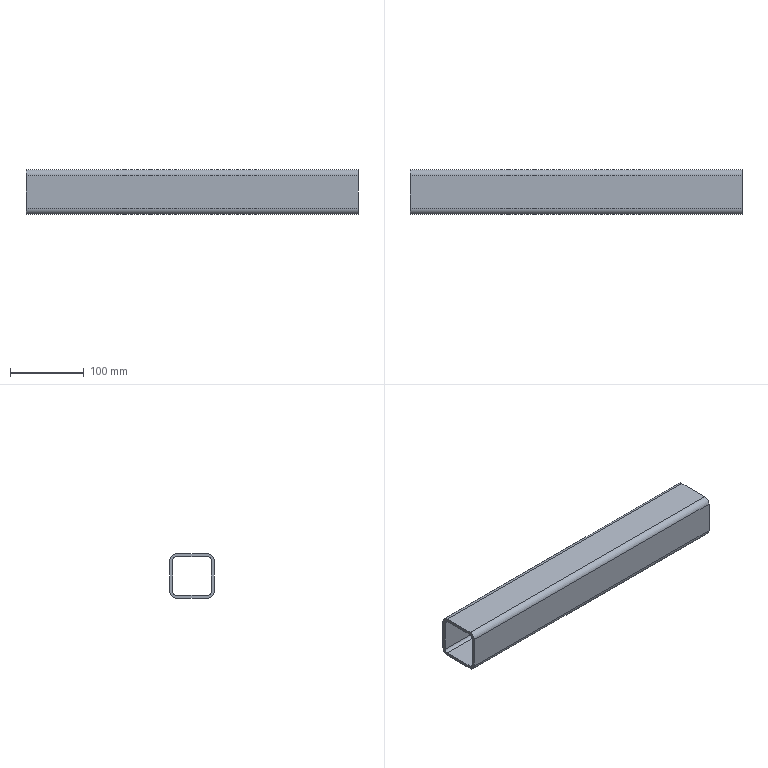Part | SolidWorks | features BaseBody 1 | 1 solid | 18 faces | box 450 x 60 x 60 mm | volume 384658 mm3 | plane 10 | cylinder 8 | commonest cylinder face diameters 8 x4 16 x4
STEP:
#1=CARTESIAN_POINT('',(210.,468.,-1308.));
#2=VERTEX_POINT('',#1);
#3=CARTESIAN_POINT('',(-240.,468.,-1308.));
#4=VERTEX_POINT('',#3);
#5=CARTESIAN_POINT('',(210.,468.,-1308.));
#6=DIRECTION('',(-1.,0.,0.));
#7=VECTOR('',#6,1000.);
#8=LINE('',#5,#7);
#9=EDGE_CURVE('',#2,#4,#8,.T.);
#10=ORIENTED_EDGE('',*,*,#9,.T.);
#11=CARTESIAN_POINT('',(-240.,468.,-1352.));
#12=VERTEX_POINT('',#11);
#13=CARTESIAN_POINT('',(-240.,468.,-1308.));
#14=DIRECTION('',(0.,0.,-1.));
#15=VECTOR('',#14,1000.);
#16=LINE('',#13,#15);
#17=EDGE_CURVE('',#4,#12,#16,.T.);
#18=ORIENTED_EDGE('',*,*,#17,.T.);
#19=CARTESIAN_POINT('',(210.,468.,-1352.));
#20=VERTEX_POINT('',#19);
#21=CARTESIAN_POINT('',(210.,468.,-1352.));
#22=DIRECTION('',(1.,0.,0.));
#23=VECTOR('',#22,1000.);
#24=LINE('',#21,#23);
#25=EDGE_CURVE('',#12,#20,#24,.T.);
#26=ORIENTED_EDGE('',*,*,#25,.T.);
#27=CARTESIAN_POINT('',(210.,468.,-1308.));
#28=DIRECTION('',(0.,0.,1.));
#29=VECTOR('',#28,1000.);
#30=LINE('',#27,#29);
#31=EDGE_CURVE('',#20,#2,#30,.T.);
#32=ORIENTED_EDGE('',*,*,#31,.T.);
#33=EDGE_LOOP('',(#10,#18,#26,#32));
#34=FACE_OUTER_BOUND('',#33,.T.);
#35=CARTESIAN_POINT('',(210.,468.,-1308.));
#36=DIRECTION('',(0.,-1.,0.));
#37=DIRECTION('',(0.,0.,-1.));
#38=AXIS2_PLACEMENT_3D('',#35,#36,#37);
#39=PLANE('',#38);
#40=ADVANCED_FACE('',(#34),#39,.T.);
#41=CARTESIAN_POINT('',(-240.,464.,-1304.));
#42=VERTEX_POINT('',#41);
#43=CARTESIAN_POINT('',(-240.,464.,-1308.));
#44=DIRECTION('',(-1.,0.,0.));
#45=DIRECTION('',(0.,0.,1.));
#46=AXIS2_PLACEMENT_3D('',#43,#44,#45);
#47=CIRCLE('',#46,4.);
#48=EDGE_CURVE('',#42,#4,#47,.T.);
#49=ORIENTED_EDGE('',*,*,#48,.F.);
#50=CARTESIAN_POINT('',(-240.,420.,-1304.));
#51=VERTEX_POINT('',#50);
#52=CARTESIAN_POINT('',(-240.,420.,-1304.));
#53=DIRECTION('',(0.,1.,0.));
#54=VECTOR('',#53,1000.);
#55=LINE('',#52,#54);
#56=EDGE_CURVE('',#51,#42,#55,.T.);
#57=ORIENTED_EDGE('',*,*,#56,.F.);
#58=CARTESIAN_POINT('',(-240.,416.,-1308.));
#59=VERTEX_POINT('',#58);
#60=CARTESIAN_POINT('',(-240.,420.,-1308.));
#61=DIRECTION('',(-1.,0.,0.));
#62=DIRECTION('',(0.,0.,1.));
#63=AXIS2_PLACEMENT_3D('',#60,#61,#62);
#64=CIRCLE('',#63,4.);
#65=EDGE_CURVE('',#59,#51,#64,.T.);
#66=ORIENTED_EDGE('',*,*,#65,.F.);
#67=CARTESIAN_POINT('',(-240.,416.,-1352.));
#68=VERTEX_POINT('',#67);
#69=CARTESIAN_POINT('',(-240.,416.,-1352.));
#70=DIRECTION('',(0.,0.,1.));
#71=VECTOR('',#70,1000.);
#72=LINE('',#69,#71);
#73=EDGE_CURVE('',#68,#59,#72,.T.);
#74=ORIENTED_EDGE('',*,*,#73,.F.);
#75=CARTESIAN_POINT('',(-240.,420.,-1356.));
#76=VERTEX_POINT('',#75);
#77=CARTESIAN_POINT('',(-240.,420.,-1352.));
#78=DIRECTION('',(-1.,0.,0.));
#79=DIRECTION('',(0.,0.,1.));
#80=AXIS2_PLACEMENT_3D('',#77,#78,#79);
#81=CIRCLE('',#80,4.);
#82=EDGE_CURVE('',#76,#68,#81,.T.);
#83=ORIENTED_EDGE('',*,*,#82,.F.);
#84=CARTESIAN_POINT('',(-240.,464.,-1356.));
#85=VERTEX_POINT('',#84);
#86=CARTESIAN_POINT('',(-240.,420.,-1356.));
#87=DIRECTION('',(0.,-1.,0.));
#88=VECTOR('',#87,1000.);
#89=LINE('',#86,#88);
#90=EDGE_CURVE('',#85,#76,#89,.T.);
#91=ORIENTED_EDGE('',*,*,#90,.F.);
#92=CARTESIAN_POINT('',(-240.,464.,-1352.));
#93=DIRECTION('',(-1.,0.,0.));
#94=DIRECTION('',(0.,0.,1.));
#95=AXIS2_PLACEMENT_3D('',#92,#93,#94);
#96=CIRCLE('',#95,4.);
#97=EDGE_CURVE('',#12,#85,#96,.T.);
#98=ORIENTED_EDGE('',*,*,#97,.F.);
#99=ORIENTED_EDGE('',*,*,#17,.F.);
#100=EDGE_LOOP('',(#49,#57,#66,#74,#83,#91,#98,#99));
#101=FACE_BOUND('',#100,.T.);
#102=CARTESIAN_POINT('',(-240.,420.,-1300.));
#103=VERTEX_POINT('',#102);
#104=CARTESIAN_POINT('',(-240.,412.,-1308.));
#105=VERTEX_POINT('',#104);
#106=CARTESIAN_POINT('',(-240.,420.,-1308.));
#107=DIRECTION('',(1.,0.,0.));
#108=DIRECTION('',(0.,0.,1.));
#109=AXIS2_PLACEMENT_3D('',#106,#107,#108);
#110=CIRCLE('',#109,8.);
#111=EDGE_CURVE('',#103,#105,#110,.T.);
#112=ORIENTED_EDGE('',*,*,#111,.F.);
#113=CARTESIAN_POINT('',(-240.,464.,-1300.));
#114=VERTEX_POINT('',#113);
#115=CARTESIAN_POINT('',(-240.,420.,-1300.));
#116=DIRECTION('',(0.,-1.,0.));
#117=VECTOR('',#116,1000.);
#118=LINE('',#115,#117);
#119=EDGE_CURVE('',#114,#103,#118,.T.);
#120=ORIENTED_EDGE('',*,*,#119,.F.);
#121=CARTESIAN_POINT('',(-240.,472.,-1308.));
#122=VERTEX_POINT('',#121);
#123=CARTESIAN_POINT('',(-240.,464.,-1308.));
#124=DIRECTION('',(1.,0.,0.));
#125=DIRECTION('',(0.,0.,1.));
#126=AXIS2_PLACEMENT_3D('',#123,#124,#125);
#127=CIRCLE('',#126,8.);
#128=EDGE_CURVE('',#122,#114,#127,.T.);
#129=ORIENTED_EDGE('',*,*,#128,.F.);
#130=CARTESIAN_POINT('',(-240.,472.,-1352.));
#131=VERTEX_POINT('',#130);
#132=CARTESIAN_POINT('',(-240.,472.,-1352.));
#133=DIRECTION('',(0.,0.,1.));
#134=VECTOR('',#133,1000.);
#135=LINE('',#132,#134);
#136=EDGE_CURVE('',#131,#122,#135,.T.);
#137=ORIENTED_EDGE('',*,*,#136,.F.);
#138=CARTESIAN_POINT('',(-240.,464.,-1360.));
#139=VERTEX_POINT('',#138);
#140=CARTESIAN_POINT('',(-240.,464.,-1352.));
#141=DIRECTION('',(1.,0.,0.));
#142=DIRECTION('',(0.,0.,1.));
#143=AXIS2_PLACEMENT_3D('',#140,#141,#142);
#144=CIRCLE('',#143,8.);
#145=EDGE_CURVE('',#139,#131,#144,.T.);
#146=ORIENTED_EDGE('',*,*,#145,.F.);
#147=CARTESIAN_POINT('',(-240.,420.,-1360.));
#148=VERTEX_POINT('',#147);
#149=CARTESIAN_POINT('',(-240.,420.,-1360.));
#150=DIRECTION('',(0.,1.,0.));
#151=VECTOR('',#150,1000.);
#152=LINE('',#149,#151);
#153=EDGE_CURVE('',#148,#139,#152,.T.);
#154=ORIENTED_EDGE('',*,*,#153,.F.);
#155=CARTESIAN_POINT('',(-240.,412.,-1352.));
#156=VERTEX_POINT('',#155);
#157=CARTESIAN_POINT('',(-240.,420.,-1352.));
#158=DIRECTION('',(1.,0.,0.));
#159=DIRECTION('',(0.,0.,1.));
#160=AXIS2_PLACEMENT_3D('',#157,#158,#159);
#161=CIRCLE('',#160,8.);
#162=EDGE_CURVE('',#156,#148,#161,.T.);
#163=ORIENTED_EDGE('',*,*,#162,.F.);
#164=CARTESIAN_POINT('',(-240.,412.,-1352.));
#165=DIRECTION('',(0.,0.,-1.));
#166=VECTOR('',#165,1000.);
#167=LINE('',#164,#166);
#168=EDGE_CURVE('',#105,#156,#167,.T.);
#169=ORIENTED_EDGE('',*,*,#168,.F.);
#170=EDGE_LOOP('',(#112,#120,#129,#137,#146,#154,#163,#169));
#171=FACE_OUTER_BOUND('',#170,.T.);
#172=CARTESIAN_POINT('',(-240.,420.,-1352.));
#173=DIRECTION('',(1.,0.,0.));
#174=DIRECTION('',(0.,0.,-1.));
#175=AXIS2_PLACEMENT_3D('',#172,#173,#174);
#176=PLANE('',#175);
#177=ADVANCED_FACE('',(#101,#171),#176,.F.);
#178=CARTESIAN_POINT('',(210.,464.,-1304.));
#179=VERTEX_POINT('',#178);
#180=CARTESIAN_POINT('',(210.,464.,-1308.));
#181=DIRECTION('',(-1.,0.,0.));
#182=DIRECTION('',(0.,0.,1.));
#183=AXIS2_PLACEMENT_3D('',#180,#181,#182);
#184=CIRCLE('',#183,4.);
#185=EDGE_CURVE('',#179,#2,#184,.T.);
#186=ORIENTED_EDGE('',*,*,#185,.F.);
#187=CARTESIAN_POINT('',(210.,464.,-1304.));
#188=DIRECTION('',(1.,0.,0.));
#189=VECTOR('',#188,1000.);
#190=LINE('',#187,#189);
#191=EDGE_CURVE('',#42,#179,#190,.T.);
#192=ORIENTED_EDGE('',*,*,#191,.F.);
#193=ORIENTED_EDGE('',*,*,#48,.T.);
#194=ORIENTED_EDGE('',*,*,#9,.F.);
#195=EDGE_LOOP('',(#186,#192,#193,#194));
#196=FACE_OUTER_BOUND('',#195,.T.);
#197=CARTESIAN_POINT('',(210.,464.,-1308.));
#198=DIRECTION('',(-1.,0.,0.));
#199=DIRECTION('',(0.,0.,1.));
#200=AXIS2_PLACEMENT_3D('',#197,#198,#199);
#201=CYLINDRICAL_SURFACE('',#200,4.);
#202=ADVANCED_FACE('',(#196),#201,.F.);
#203=ORIENTED_EDGE('',*,*,#31,.F.);
#204=CARTESIAN_POINT('',(210.,464.,-1356.));
#205=VERTEX_POINT('',#204);
#206=CARTESIAN_POINT('',(210.,464.,-1352.));
#207=DIRECTION('',(-1.,0.,0.));
#208=DIRECTION('',(0.,0.,1.));
#209=AXIS2_PLACEMENT_3D('',#206,#207,#208);
#210=CIRCLE('',#209,4.);
#211=EDGE_CURVE('',#20,#205,#210,.T.);
#212=ORIENTED_EDGE('',*,*,#211,.T.);
#213=CARTESIAN_POINT('',(210.,420.,-1356.));
#214=VERTEX_POINT('',#213);
#215=CARTESIAN_POINT('',(210.,420.,-1356.));
#216=DIRECTION('',(0.,-1.,0.));
#217=VECTOR('',#216,1000.);
#218=LINE('',#215,#217);
#219=EDGE_CURVE('',#205,#214,#218,.T.);
#220=ORIENTED_EDGE('',*,*,#219,.T.);
#221=CARTESIAN_POINT('',(210.,416.,-1352.));
#222=VERTEX_POINT('',#221);
#223=CARTESIAN_POINT('',(210.,420.,-1352.));
#224=DIRECTION('',(-1.,0.,0.));
#225=DIRECTION('',(0.,0.,1.));
#226=AXIS2_PLACEMENT_3D('',#223,#224,#225);
#227=CIRCLE('',#226,4.);
#228=EDGE_CURVE('',#214,#222,#227,.T.);
#229=ORIENTED_EDGE('',*,*,#228,.T.);
#230=CARTESIAN_POINT('',(210.,416.,-1308.));
#231=VERTEX_POINT('',#230);
#232=CARTESIAN_POINT('',(210.,416.,-1352.));
#233=DIRECTION('',(0.,0.,1.));
#234=VECTOR('',#233,1000.);
#235=LINE('',#232,#234);
#236=EDGE_CURVE('',#222,#231,#235,.T.);
#237=ORIENTED_EDGE('',*,*,#236,.T.);
#238=CARTESIAN_POINT('',(210.,420.,-1304.));
#239=VERTEX_POINT('',#238);
#240=CARTESIAN_POINT('',(210.,420.,-1308.));
#241=DIRECTION('',(-1.,0.,0.));
#242=DIRECTION('',(0.,0.,1.));
#243=AXIS2_PLACEMENT_3D('',#240,#241,#242);
#244=CIRCLE('',#243,4.);
#245=EDGE_CURVE('',#231,#239,#244,.T.);
#246=ORIENTED_EDGE('',*,*,#245,.T.);
#247=CARTESIAN_POINT('',(210.,420.,-1304.));
#248=DIRECTION('',(0.,1.,0.));
#249=VECTOR('',#248,1000.);
#250=LINE('',#247,#249);
#251=EDGE_CURVE('',#239,#179,#250,.T.);
#252=ORIENTED_EDGE('',*,*,#251,.T.);
#253=ORIENTED_EDGE('',*,*,#185,.T.);
#254=EDGE_LOOP('',(#203,#212,#220,#229,#237,#246,#252,#253));
#255=FACE_BOUND('',#254,.T.);
#256=CARTESIAN_POINT('',(210.,412.,-1308.));
#257=VERTEX_POINT('',#256);
#258=CARTESIAN_POINT('',(210.,412.,-1352.));
#259=VERTEX_POINT('',#258);
#260=CARTESIAN_POINT('',(210.,412.,-1352.));
#261=DIRECTION('',(0.,0.,-1.));
#262=VECTOR('',#261,1000.);
#263=LINE('',#260,#262);
#264=EDGE_CURVE('',#257,#259,#263,.T.);
#265=ORIENTED_EDGE('',*,*,#264,.T.);
#266=CARTESIAN_POINT('',(210.,420.,-1360.));
#267=VERTEX_POINT('',#266);
#268=CARTESIAN_POINT('',(210.,420.,-1352.));
#269=DIRECTION('',(1.,0.,0.));
#270=DIRECTION('',(0.,0.,1.));
#271=AXIS2_PLACEMENT_3D('',#268,#269,#270);
#272=CIRCLE('',#271,8.);
#273=EDGE_CURVE('',#259,#267,#272,.T.);
#274=ORIENTED_EDGE('',*,*,#273,.T.);
#275=CARTESIAN_POINT('',(210.,464.,-1360.));
#276=VERTEX_POINT('',#275);
#277=CARTESIAN_POINT('',(210.,420.,-1360.));
#278=DIRECTION('',(0.,1.,0.));
#279=VECTOR('',#278,1000.);
#280=LINE('',#277,#279);
#281=EDGE_CURVE('',#267,#276,#280,.T.);
#282=ORIENTED_EDGE('',*,*,#281,.T.);
#283=CARTESIAN_POINT('',(210.,472.,-1352.));
#284=VERTEX_POINT('',#283);
#285=CARTESIAN_POINT('',(210.,464.,-1352.));
#286=DIRECTION('',(1.,0.,0.));
#287=DIRECTION('',(0.,0.,1.));
#288=AXIS2_PLACEMENT_3D('',#285,#286,#287);
#289=CIRCLE('',#288,8.);
#290=EDGE_CURVE('',#276,#284,#289,.T.);
#291=ORIENTED_EDGE('',*,*,#290,.T.);
#292=CARTESIAN_POINT('',(210.,472.,-1308.));
#293=VERTEX_POINT('',#292);
#294=CARTESIAN_POINT('',(210.,472.,-1352.));
#295=DIRECTION('',(0.,0.,1.));
#296=VECTOR('',#295,1000.);
#297=LINE('',#294,#296);
#298=EDGE_CURVE('',#284,#293,#297,.T.);
#299=ORIENTED_EDGE('',*,*,#298,.T.);
#300=CARTESIAN_POINT('',(210.,464.,-1300.));
#301=VERTEX_POINT('',#300);
#302=CARTESIAN_POINT('',(210.,464.,-1308.));
#303=DIRECTION('',(1.,0.,0.));
#304=DIRECTION('',(0.,0.,1.));
#305=AXIS2_PLACEMENT_3D('',#302,#303,#304);
#306=CIRCLE('',#305,8.);
#307=EDGE_CURVE('',#293,#301,#306,.T.);
#308=ORIENTED_EDGE('',*,*,#307,.T.);
#309=CARTESIAN_POINT('',(210.,420.,-1300.));
#310=VERTEX_POINT('',#309);
#311=CARTESIAN_POINT('',(210.,420.,-1300.));
#312=DIRECTION('',(0.,-1.,0.));
#313=VECTOR('',#312,1000.);
#314=LINE('',#311,#313);
#315=EDGE_CURVE('',#301,#310,#314,.T.);
#316=ORIENTED_EDGE('',*,*,#315,.T.);
#317=CARTESIAN_POINT('',(210.,420.,-1308.));
#318=DIRECTION('',(1.,0.,0.));
#319=DIRECTION('',(0.,0.,1.));
#320=AXIS2_PLACEMENT_3D('',#317,#318,#319);
#321=CIRCLE('',#320,8.);
#322=EDGE_CURVE('',#310,#257,#321,.T.);
#323=ORIENTED_EDGE('',*,*,#322,.T.);
#324=EDGE_LOOP('',(#265,#274,#282,#291,#299,#308,#316,#323));
#325=FACE_OUTER_BOUND('',#324,.T.);
#326=CARTESIAN_POINT('',(210.,420.,-1352.));
#327=DIRECTION('',(1.,0.,0.));
#328=DIRECTION('',(0.,0.,-1.));
#329=AXIS2_PLACEMENT_3D('',#326,#327,#328);
#330=PLANE('',#329);
#331=ADVANCED_FACE('',(#255,#325),#330,.T.);
#332=ORIENTED_EDGE('',*,*,#211,.F.);
#333=ORIENTED_EDGE('',*,*,#25,.F.);
#334=ORIENTED_EDGE('',*,*,#97,.T.);
#335=CARTESIAN_POINT('',(210.,464.,-1356.));
#336=DIRECTION('',(-1.,0.,0.));
#337=VECTOR('',#336,1000.);
#338=LINE('',#335,#337);
#339=EDGE_CURVE('',#205,#85,#338,.T.);
#340=ORIENTED_EDGE('',*,*,#339,.F.);
#341=EDGE_LOOP('',(#332,#333,#334,#340));
#342=FACE_OUTER_BOUND('',#341,.T.);
#343=CARTESIAN_POINT('',(210.,464.,-1352.));
#344=DIRECTION('',(-1.,0.,0.));
#345=DIRECTION('',(0.,0.,1.));
#346=AXIS2_PLACEMENT_3D('',#343,#344,#345);
#347=CYLINDRICAL_SURFACE('',#346,4.);
#348=ADVANCED_FACE('',(#342),#347,.F.);
#349=CARTESIAN_POINT('',(210.,420.,-1304.));
#350=DIRECTION('',(-1.,0.,0.));
#351=VECTOR('',#350,1000.);
#352=LINE('',#349,#351);
#353=EDGE_CURVE('',#239,#51,#352,.T.);
#354=ORIENTED_EDGE('',*,*,#353,.T.);
#355=ORIENTED_EDGE('',*,*,#56,.T.);
#356=ORIENTED_EDGE('',*,*,#191,.T.);
#357=ORIENTED_EDGE('',*,*,#251,.F.);
#358=EDGE_LOOP('',(#354,#355,#356,#357));
#359=FACE_OUTER_BOUND('',#358,.T.);
#360=CARTESIAN_POINT('',(210.,464.,-1304.));
#361=DIRECTION('',(0.,0.,-1.));
#362=DIRECTION('',(-1.,0.,0.));
#363=AXIS2_PLACEMENT_3D('',#360,#361,#362);
#364=PLANE('',#363);
#365=ADVANCED_FACE('',(#359),#364,.T.);
#366=ORIENTED_EDGE('',*,*,#245,.F.);
#367=CARTESIAN_POINT('',(210.,416.,-1308.));
#368=DIRECTION('',(1.,0.,0.));
#369=VECTOR('',#368,1000.);
#370=LINE('',#367,#369);
#371=EDGE_CURVE('',#59,#231,#370,.T.);
#372=ORIENTED_EDGE('',*,*,#371,.F.);
#373=ORIENTED_EDGE('',*,*,#65,.T.);
#374=ORIENTED_EDGE('',*,*,#353,.F.);
#375=EDGE_LOOP('',(#366,#372,#373,#374));
#376=FACE_OUTER_BOUND('',#375,.T.);
#377=CARTESIAN_POINT('',(210.,420.,-1308.));
#378=DIRECTION('',(-1.,0.,0.));
#379=DIRECTION('',(0.,0.,1.));
#380=AXIS2_PLACEMENT_3D('',#377,#378,#379);
#381=CYLINDRICAL_SURFACE('',#380,4.);
#382=ADVANCED_FACE('',(#376),#381,.F.);
#383=CARTESIAN_POINT('',(210.,416.,-1352.));
#384=DIRECTION('',(-1.,0.,0.));
#385=VECTOR('',#384,1000.);
#386=LINE('',#383,#385);
#387=EDGE_CURVE('',#222,#68,#386,.T.);
#388=ORIENTED_EDGE('',*,*,#387,.T.);
#389=ORIENTED_EDGE('',*,*,#73,.T.);
#390=ORIENTED_EDGE('',*,*,#371,.T.);
#391=ORIENTED_EDGE('',*,*,#236,.F.);
#392=EDGE_LOOP('',(#388,#389,#390,#391));
#393=FACE_OUTER_BOUND('',#392,.T.);
#394=CARTESIAN_POINT('',(210.,416.,-1352.));
#395=DIRECTION('',(0.,1.,0.));
#396=DIRECTION('',(0.,0.,1.));
#397=AXIS2_PLACEMENT_3D('',#394,#395,#396);
#398=PLANE('',#397);
#399=ADVANCED_FACE('',(#393),#398,.T.);
#400=ORIENTED_EDGE('',*,*,#228,.F.);
#401=CARTESIAN_POINT('',(210.,420.,-1356.));
#402=DIRECTION('',(1.,0.,0.));
#403=VECTOR('',#402,1000.);
#404=LINE('',#401,#403);
#405=EDGE_CURVE('',#76,#214,#404,.T.);
#406=ORIENTED_EDGE('',*,*,#405,.F.);
#407=ORIENTED_EDGE('',*,*,#82,.T.);
#408=ORIENTED_EDGE('',*,*,#387,.F.);
#409=EDGE_LOOP('',(#400,#406,#407,#408));
#410=FACE_OUTER_BOUND('',#409,.T.);
#411=CARTESIAN_POINT('',(210.,420.,-1352.));
#412=DIRECTION('',(-1.,0.,0.));
#413=DIRECTION('',(0.,0.,1.));
#414=AXIS2_PLACEMENT_3D('',#411,#412,#413);
#415=CYLINDRICAL_SURFACE('',#414,4.);
#416=ADVANCED_FACE('',(#410),#415,.F.);
#417=ORIENTED_EDGE('',*,*,#339,.T.);
#418=ORIENTED_EDGE('',*,*,#90,.T.);
#419=ORIENTED_EDGE('',*,*,#405,.T.);
#420=ORIENTED_EDGE('',*,*,#219,.F.);
#421=EDGE_LOOP('',(#417,#418,#419,#420));
#422=FACE_OUTER_BOUND('',#421,.T.);
#423=CARTESIAN_POINT('',(210.,420.,-1356.));
#424=DIRECTION('',(0.,0.,1.));
#425=DIRECTION('',(1.,0.,0.));
#426=AXIS2_PLACEMENT_3D('',#423,#424,#425);
#427=PLANE('',#426);
#428=ADVANCED_FACE('',(#422),#427,.T.);
#429=ORIENTED_EDGE('',*,*,#264,.F.);
#430=CARTESIAN_POINT('',(210.,412.,-1308.));
#431=DIRECTION('',(1.,0.,0.));
#432=VECTOR('',#431,1000.);
#433=LINE('',#430,#432);
#434=EDGE_CURVE('',#105,#257,#433,.T.);
#435=ORIENTED_EDGE('',*,*,#434,.F.);
#436=ORIENTED_EDGE('',*,*,#168,.T.);
#437=CARTESIAN_POINT('',(210.,412.,-1352.));
#438=DIRECTION('',(-1.,0.,0.));
#439=VECTOR('',#438,1000.);
#440=LINE('',#437,#439);
#441=EDGE_CURVE('',#259,#156,#440,.T.);
#442=ORIENTED_EDGE('',*,*,#441,.F.);
#443=EDGE_LOOP('',(#429,#435,#436,#442));
#444=FACE_OUTER_BOUND('',#443,.T.);
#445=CARTESIAN_POINT('',(210.,412.,-1352.));
#446=DIRECTION('',(0.,1.,0.));
#447=DIRECTION('',(0.,0.,1.));
#448=AXIS2_PLACEMENT_3D('',#445,#446,#447);
#449=PLANE('',#448);
#450=ADVANCED_FACE('',(#444),#449,.F.);
#451=CARTESIAN_POINT('',(210.,420.,-1300.));
#452=DIRECTION('',(-1.,0.,0.));
#453=VECTOR('',#452,1000.);
#454=LINE('',#451,#453);
#455=EDGE_CURVE('',#310,#103,#454,.T.);
#456=ORIENTED_EDGE('',*,*,#455,.T.);
#457=ORIENTED_EDGE('',*,*,#111,.T.);
#458=ORIENTED_EDGE('',*,*,#434,.T.);
#459=ORIENTED_EDGE('',*,*,#322,.F.);
#460=EDGE_LOOP('',(#456,#457,#458,#459));
#461=FACE_OUTER_BOUND('',#460,.T.);
#462=CARTESIAN_POINT('',(210.,420.,-1308.));
#463=DIRECTION('',(-1.,0.,0.));
#464=DIRECTION('',(0.,0.,1.));
#465=AXIS2_PLACEMENT_3D('',#462,#463,#464);
#466=CYLINDRICAL_SURFACE('',#465,8.);
#467=ADVANCED_FACE('',(#461),#466,.T.);
#468=ORIENTED_EDGE('',*,*,#315,.F.);
#469=CARTESIAN_POINT('',(210.,464.,-1300.));
#470=DIRECTION('',(1.,0.,0.));
#471=VECTOR('',#470,1000.);
#472=LINE('',#469,#471);
#473=EDGE_CURVE('',#114,#301,#472,.T.);
#474=ORIENTED_EDGE('',*,*,#473,.F.);
#475=ORIENTED_EDGE('',*,*,#119,.T.);
#476=ORIENTED_EDGE('',*,*,#455,.F.);
#477=EDGE_LOOP('',(#468,#474,#475,#476));
#478=FACE_OUTER_BOUND('',#477,.T.);
#479=CARTESIAN_POINT('',(210.,464.,-1300.));
#480=DIRECTION('',(0.,0.,-1.));
#481=DIRECTION('',(-1.,0.,0.));
#482=AXIS2_PLACEMENT_3D('',#479,#480,#481);
#483=PLANE('',#482);
#484=ADVANCED_FACE('',(#478),#483,.F.);
#485=CARTESIAN_POINT('',(210.,472.,-1308.));
#486=DIRECTION('',(-1.,0.,0.));
#487=VECTOR('',#486,1000.);
#488=LINE('',#485,#487);
#489=EDGE_CURVE('',#293,#122,#488,.T.);
#490=ORIENTED_EDGE('',*,*,#489,.T.);
#491=ORIENTED_EDGE('',*,*,#128,.T.);
#492=ORIENTED_EDGE('',*,*,#473,.T.);
#493=ORIENTED_EDGE('',*,*,#307,.F.);
#494=EDGE_LOOP('',(#490,#491,#492,#493));
#495=FACE_OUTER_BOUND('',#494,.T.);
#496=CARTESIAN_POINT('',(210.,464.,-1308.));
#497=DIRECTION('',(-1.,0.,0.));
#498=DIRECTION('',(0.,0.,1.));
#499=AXIS2_PLACEMENT_3D('',#496,#497,#498);
#500=CYLINDRICAL_SURFACE('',#499,8.);
#501=ADVANCED_FACE('',(#495),#500,.T.);
#502=ORIENTED_EDGE('',*,*,#298,.F.);
#503=CARTESIAN_POINT('',(210.,472.,-1352.));
#504=DIRECTION('',(1.,0.,0.));
#505=VECTOR('',#504,1000.);
#506=LINE('',#503,#505);
#507=EDGE_CURVE('',#131,#284,#506,.T.);
#508=ORIENTED_EDGE('',*,*,#507,.F.);
#509=ORIENTED_EDGE('',*,*,#136,.T.);
#510=ORIENTED_EDGE('',*,*,#489,.F.);
#511=EDGE_LOOP('',(#502,#508,#509,#510));
#512=FACE_OUTER_BOUND('',#511,.T.);
#513=CARTESIAN_POINT('',(210.,472.,-1308.));
#514=DIRECTION('',(0.,-1.,0.));
#515=DIRECTION('',(0.,0.,-1.));
#516=AXIS2_PLACEMENT_3D('',#513,#514,#515);
#517=PLANE('',#516);
#518=ADVANCED_FACE('',(#512),#517,.F.);
#519=CARTESIAN_POINT('',(210.,464.,-1360.));
#520=DIRECTION('',(-1.,0.,0.));
#521=VECTOR('',#520,1000.);
#522=LINE('',#519,#521);
#523=EDGE_CURVE('',#276,#139,#522,.T.);
#524=ORIENTED_EDGE('',*,*,#523,.T.);
#525=ORIENTED_EDGE('',*,*,#145,.T.);
#526=ORIENTED_EDGE('',*,*,#507,.T.);
#527=ORIENTED_EDGE('',*,*,#290,.F.);
#528=EDGE_LOOP('',(#524,#525,#526,#527));
#529=FACE_OUTER_BOUND('',#528,.T.);
#530=CARTESIAN_POINT('',(210.,464.,-1352.));
#531=DIRECTION('',(-1.,0.,0.));
#532=DIRECTION('',(0.,0.,1.));
#533=AXIS2_PLACEMENT_3D('',#530,#531,#532);
#534=CYLINDRICAL_SURFACE('',#533,8.);
#535=ADVANCED_FACE('',(#529),#534,.T.);
#536=ORIENTED_EDGE('',*,*,#281,.F.);
#537=CARTESIAN_POINT('',(210.,420.,-1360.));
#538=DIRECTION('',(1.,0.,0.));
#539=VECTOR('',#538,1000.);
#540=LINE('',#537,#539);
#541=EDGE_CURVE('',#148,#267,#540,.T.);
#542=ORIENTED_EDGE('',*,*,#541,.F.);
#543=ORIENTED_EDGE('',*,*,#153,.T.);
#544=ORIENTED_EDGE('',*,*,#523,.F.);
#545=EDGE_LOOP('',(#536,#542,#543,#544));
#546=FACE_OUTER_BOUND('',#545,.T.);
#547=CARTESIAN_POINT('',(210.,420.,-1360.));
#548=DIRECTION('',(0.,0.,1.));
#549=DIRECTION('',(1.,0.,0.));
#550=AXIS2_PLACEMENT_3D('',#547,#548,#549);
#551=PLANE('',#550);
#552=ADVANCED_FACE('',(#546),#551,.F.);
#553=ORIENTED_EDGE('',*,*,#441,.T.);
#554=ORIENTED_EDGE('',*,*,#162,.T.);
#555=ORIENTED_EDGE('',*,*,#541,.T.);
#556=ORIENTED_EDGE('',*,*,#273,.F.);
#557=EDGE_LOOP('',(#553,#554,#555,#556));
#558=FACE_OUTER_BOUND('',#557,.T.);
#559=CARTESIAN_POINT('',(210.,420.,-1352.));
#560=DIRECTION('',(-1.,0.,0.));
#561=DIRECTION('',(0.,0.,1.));
#562=AXIS2_PLACEMENT_3D('',#559,#560,#561);
#563=CYLINDRICAL_SURFACE('',#562,8.);
#564=ADVANCED_FACE('',(#558),#563,.T.);
#565=CLOSED_SHELL('',(#40,#177,#202,#331,#348,#365,#382,#399,#416,#428,#450,#467,#484,#501,#518,#535,#552,#564));
#566=MANIFOLD_SOLID_BREP('',#565);
#567=CARTESIAN_POINT('',(0.,0.,0.));
#568=DIRECTION('',(0.,0.,1.));
#569=DIRECTION('',(1.,0.,0.));
#570=AXIS2_PLACEMENT_3D('',#567,#568,#569);
#571=(LENGTH_UNIT()NAMED_UNIT(*)SI_UNIT(.MILLI.,.METRE.));
#572=UNCERTAINTY_MEASURE_WITH_UNIT(LENGTH_MEASURE(0.00001),#571,'','');
#573=(NAMED_UNIT(*)PLANE_ANGLE_UNIT()SI_UNIT($,.RADIAN.));
#574=(NAMED_UNIT(*)SI_UNIT($,.STERADIAN.)SOLID_ANGLE_UNIT());
#575=(GEOMETRIC_REPRESENTATION_CONTEXT(3)GLOBAL_UNCERTAINTY_ASSIGNED_CONTEXT((#572))GLOBAL_UNIT_ASSIGNED_CONTEXT((#571,#573,#574))REPRESENTATION_CONTEXT('',''));
#576=ADVANCED_BREP_SHAPE_REPRESENTATION('',(#566,#570),#575);